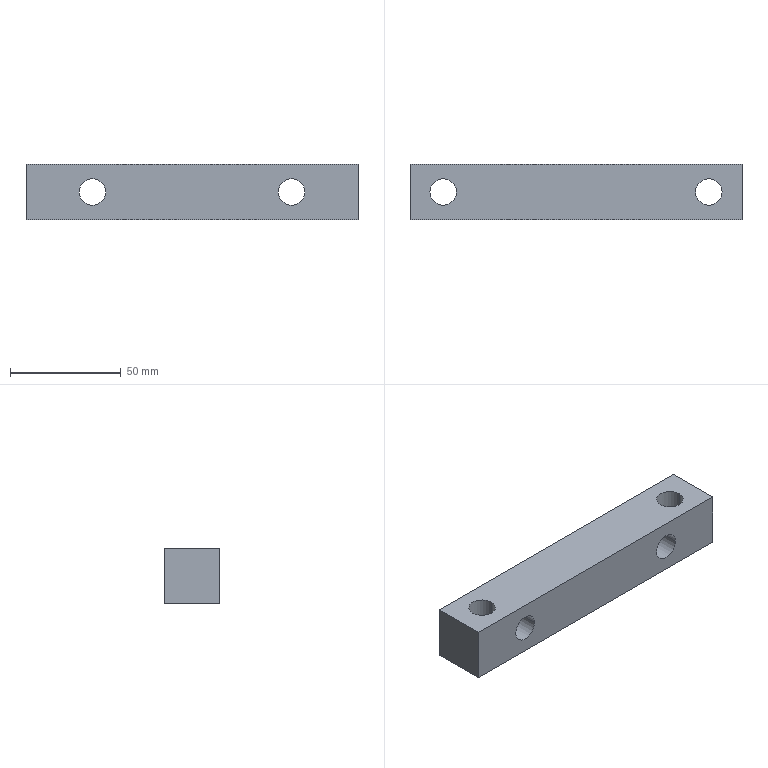Part | STEP file | J013-EBZ05-14-06-Part-1 | 1 solid | 14 faces | box 150 x 25 x 25 mm | volume 82440 mm3 | cylinder 8 | plane 6 | commonest cylinder face diameters 12 x8
STEP:
#1=CARTESIAN_POINT('',(114.,25.,12.5));
#2=VERTEX_POINT('',#1);
#3=CARTESIAN_POINT('',(126.,25.,12.5));
#4=VERTEX_POINT('',#3);
#5=CARTESIAN_POINT('',(120.,25.,12.5));
#6=DIRECTION('',(0.,-1.,0.));
#7=DIRECTION('',(1.,0.,0.));
#8=AXIS2_PLACEMENT_3D('',#5,#6,#7);
#9=CIRCLE('',#8,6.);
#10=EDGE_CURVE('',#2,#4,#9,.T.);
#11=ORIENTED_EDGE('',*,*,#10,.F.);
#12=CARTESIAN_POINT('',(114.,0.,12.5));
#13=VERTEX_POINT('',#12);
#14=CARTESIAN_POINT('',(114.,25.,12.5));
#15=DIRECTION('',(0.,-1.,0.));
#16=VECTOR('',#15,1000.);
#17=LINE('',#14,#16);
#18=EDGE_CURVE('',#2,#13,#17,.T.);
#19=ORIENTED_EDGE('',*,*,#18,.T.);
#20=CARTESIAN_POINT('',(126.,0.,12.5));
#21=VERTEX_POINT('',#20);
#22=CARTESIAN_POINT('',(120.,0.,12.5));
#23=DIRECTION('',(0.,1.,0.));
#24=DIRECTION('',(-1.,0.,0.));
#25=AXIS2_PLACEMENT_3D('',#22,#23,#24);
#26=CIRCLE('',#25,6.);
#27=EDGE_CURVE('',#21,#13,#26,.T.);
#28=ORIENTED_EDGE('',*,*,#27,.F.);
#29=CARTESIAN_POINT('',(126.,25.,12.5));
#30=DIRECTION('',(0.,-1.,0.));
#31=VECTOR('',#30,1000.);
#32=LINE('',#29,#31);
#33=EDGE_CURVE('',#4,#21,#32,.T.);
#34=ORIENTED_EDGE('',*,*,#33,.F.);
#35=EDGE_LOOP('',(#11,#19,#28,#34));
#36=FACE_OUTER_BOUND('',#35,.T.);
#37=CARTESIAN_POINT('',(120.,25.,12.5));
#38=DIRECTION('',(0.,-1.,0.));
#39=DIRECTION('',(1.,0.,0.));
#40=AXIS2_PLACEMENT_3D('',#37,#38,#39);
#41=CYLINDRICAL_SURFACE('',#40,6.);
#42=ADVANCED_FACE('',(#36),#41,.F.);
#43=CARTESIAN_POINT('',(129.,12.5,25.));
#44=VERTEX_POINT('',#43);
#45=CARTESIAN_POINT('',(141.,12.5,25.));
#46=VERTEX_POINT('',#45);
#47=CARTESIAN_POINT('',(135.,12.5,25.));
#48=DIRECTION('',(0.,0.,-1.));
#49=DIRECTION('',(1.,0.,0.));
#50=AXIS2_PLACEMENT_3D('',#47,#48,#49);
#51=CIRCLE('',#50,6.);
#52=EDGE_CURVE('',#44,#46,#51,.T.);
#53=ORIENTED_EDGE('',*,*,#52,.F.);
#54=CARTESIAN_POINT('',(129.,12.5,0.));
#55=VERTEX_POINT('',#54);
#56=CARTESIAN_POINT('',(129.,12.5,25.));
#57=DIRECTION('',(0.,0.,-1.));
#58=VECTOR('',#57,1000.);
#59=LINE('',#56,#58);
#60=EDGE_CURVE('',#44,#55,#59,.T.);
#61=ORIENTED_EDGE('',*,*,#60,.T.);
#62=CARTESIAN_POINT('',(141.,12.5,0.));
#63=VERTEX_POINT('',#62);
#64=CARTESIAN_POINT('',(135.,12.5,0.));
#65=DIRECTION('',(0.,0.,1.));
#66=DIRECTION('',(-1.,0.,0.));
#67=AXIS2_PLACEMENT_3D('',#64,#65,#66);
#68=CIRCLE('',#67,6.);
#69=EDGE_CURVE('',#63,#55,#68,.T.);
#70=ORIENTED_EDGE('',*,*,#69,.F.);
#71=CARTESIAN_POINT('',(141.,12.5,25.));
#72=DIRECTION('',(0.,0.,-1.));
#73=VECTOR('',#72,1000.);
#74=LINE('',#71,#73);
#75=EDGE_CURVE('',#46,#63,#74,.T.);
#76=ORIENTED_EDGE('',*,*,#75,.F.);
#77=EDGE_LOOP('',(#53,#61,#70,#76));
#78=FACE_OUTER_BOUND('',#77,.T.);
#79=CARTESIAN_POINT('',(135.,12.5,25.));
#80=DIRECTION('',(0.,0.,-1.));
#81=DIRECTION('',(1.,0.,0.));
#82=AXIS2_PLACEMENT_3D('',#79,#80,#81);
#83=CYLINDRICAL_SURFACE('',#82,6.);
#84=ADVANCED_FACE('',(#78),#83,.F.);
#85=CARTESIAN_POINT('',(9.,12.5,25.));
#86=VERTEX_POINT('',#85);
#87=CARTESIAN_POINT('',(21.,12.5,25.));
#88=VERTEX_POINT('',#87);
#89=CARTESIAN_POINT('',(15.,12.5,25.));
#90=DIRECTION('',(0.,0.,-1.));
#91=DIRECTION('',(1.,0.,0.));
#92=AXIS2_PLACEMENT_3D('',#89,#90,#91);
#93=CIRCLE('',#92,6.);
#94=EDGE_CURVE('',#86,#88,#93,.T.);
#95=ORIENTED_EDGE('',*,*,#94,.F.);
#96=CARTESIAN_POINT('',(9.,12.5,0.));
#97=VERTEX_POINT('',#96);
#98=CARTESIAN_POINT('',(9.,12.5,25.));
#99=DIRECTION('',(0.,0.,-1.));
#100=VECTOR('',#99,1000.);
#101=LINE('',#98,#100);
#102=EDGE_CURVE('',#86,#97,#101,.T.);
#103=ORIENTED_EDGE('',*,*,#102,.T.);
#104=CARTESIAN_POINT('',(21.,12.5,0.));
#105=VERTEX_POINT('',#104);
#106=CARTESIAN_POINT('',(15.,12.5,0.));
#107=DIRECTION('',(0.,0.,1.));
#108=DIRECTION('',(-1.,0.,0.));
#109=AXIS2_PLACEMENT_3D('',#106,#107,#108);
#110=CIRCLE('',#109,6.);
#111=EDGE_CURVE('',#105,#97,#110,.T.);
#112=ORIENTED_EDGE('',*,*,#111,.F.);
#113=CARTESIAN_POINT('',(21.,12.5,25.));
#114=DIRECTION('',(0.,0.,-1.));
#115=VECTOR('',#114,1000.);
#116=LINE('',#113,#115);
#117=EDGE_CURVE('',#88,#105,#116,.T.);
#118=ORIENTED_EDGE('',*,*,#117,.F.);
#119=EDGE_LOOP('',(#95,#103,#112,#118));
#120=FACE_OUTER_BOUND('',#119,.T.);
#121=CARTESIAN_POINT('',(15.,12.5,25.));
#122=DIRECTION('',(0.,0.,-1.));
#123=DIRECTION('',(1.,0.,0.));
#124=AXIS2_PLACEMENT_3D('',#121,#122,#123);
#125=CYLINDRICAL_SURFACE('',#124,6.);
#126=ADVANCED_FACE('',(#120),#125,.F.);
#127=CARTESIAN_POINT('',(24.,25.,12.5));
#128=VERTEX_POINT('',#127);
#129=CARTESIAN_POINT('',(36.,25.,12.5));
#130=VERTEX_POINT('',#129);
#131=CARTESIAN_POINT('',(30.,25.,12.5));
#132=DIRECTION('',(0.,-1.,0.));
#133=DIRECTION('',(1.,0.,0.));
#134=AXIS2_PLACEMENT_3D('',#131,#132,#133);
#135=CIRCLE('',#134,6.);
#136=EDGE_CURVE('',#128,#130,#135,.T.);
#137=ORIENTED_EDGE('',*,*,#136,.F.);
#138=CARTESIAN_POINT('',(24.,0.,12.5));
#139=VERTEX_POINT('',#138);
#140=CARTESIAN_POINT('',(24.,25.,12.5));
#141=DIRECTION('',(0.,-1.,0.));
#142=VECTOR('',#141,1000.);
#143=LINE('',#140,#142);
#144=EDGE_CURVE('',#128,#139,#143,.T.);
#145=ORIENTED_EDGE('',*,*,#144,.T.);
#146=CARTESIAN_POINT('',(36.,0.,12.5));
#147=VERTEX_POINT('',#146);
#148=CARTESIAN_POINT('',(30.,0.,12.5));
#149=DIRECTION('',(0.,1.,0.));
#150=DIRECTION('',(-1.,0.,0.));
#151=AXIS2_PLACEMENT_3D('',#148,#149,#150);
#152=CIRCLE('',#151,6.);
#153=EDGE_CURVE('',#147,#139,#152,.T.);
#154=ORIENTED_EDGE('',*,*,#153,.F.);
#155=CARTESIAN_POINT('',(36.,25.,12.5));
#156=DIRECTION('',(0.,-1.,0.));
#157=VECTOR('',#156,1000.);
#158=LINE('',#155,#157);
#159=EDGE_CURVE('',#130,#147,#158,.T.);
#160=ORIENTED_EDGE('',*,*,#159,.F.);
#161=EDGE_LOOP('',(#137,#145,#154,#160));
#162=FACE_OUTER_BOUND('',#161,.T.);
#163=CARTESIAN_POINT('',(30.,25.,12.5));
#164=DIRECTION('',(0.,-1.,0.));
#165=DIRECTION('',(1.,0.,0.));
#166=AXIS2_PLACEMENT_3D('',#163,#164,#165);
#167=CYLINDRICAL_SURFACE('',#166,6.);
#168=ADVANCED_FACE('',(#162),#167,.F.);
#169=CARTESIAN_POINT('',(135.,12.5,25.));
#170=DIRECTION('',(0.,0.,-1.));
#171=DIRECTION('',(1.,0.,0.));
#172=AXIS2_PLACEMENT_3D('',#169,#170,#171);
#173=CIRCLE('',#172,6.);
#174=EDGE_CURVE('',#46,#44,#173,.T.);
#175=ORIENTED_EDGE('',*,*,#174,.T.);
#176=ORIENTED_EDGE('',*,*,#52,.T.);
#177=EDGE_LOOP('',(#175,#176));
#178=FACE_BOUND('',#177,.T.);
#179=CARTESIAN_POINT('',(15.,12.5,25.));
#180=DIRECTION('',(0.,0.,-1.));
#181=DIRECTION('',(1.,0.,0.));
#182=AXIS2_PLACEMENT_3D('',#179,#180,#181);
#183=CIRCLE('',#182,6.);
#184=EDGE_CURVE('',#88,#86,#183,.T.);
#185=ORIENTED_EDGE('',*,*,#184,.T.);
#186=ORIENTED_EDGE('',*,*,#94,.T.);
#187=EDGE_LOOP('',(#185,#186));
#188=FACE_BOUND('',#187,.T.);
#189=CARTESIAN_POINT('',(0.,25.,25.));
#190=VERTEX_POINT('',#189);
#191=CARTESIAN_POINT('',(150.,25.,25.));
#192=VERTEX_POINT('',#191);
#193=CARTESIAN_POINT('',(75.,25.,25.));
#194=DIRECTION('',(1.,0.,0.));
#195=VECTOR('',#194,1000.);
#196=LINE('',#193,#195);
#197=EDGE_CURVE('',#190,#192,#196,.T.);
#198=ORIENTED_EDGE('',*,*,#197,.F.);
#199=CARTESIAN_POINT('',(0.,0.,25.));
#200=VERTEX_POINT('',#199);
#201=CARTESIAN_POINT('',(0.,12.5,25.));
#202=DIRECTION('',(0.,1.,0.));
#203=VECTOR('',#202,1000.);
#204=LINE('',#201,#203);
#205=EDGE_CURVE('',#200,#190,#204,.T.);
#206=ORIENTED_EDGE('',*,*,#205,.F.);
#207=CARTESIAN_POINT('',(150.,0.,25.));
#208=VERTEX_POINT('',#207);
#209=CARTESIAN_POINT('',(75.,0.,25.));
#210=DIRECTION('',(-1.,0.,0.));
#211=VECTOR('',#210,1000.);
#212=LINE('',#209,#211);
#213=EDGE_CURVE('',#208,#200,#212,.T.);
#214=ORIENTED_EDGE('',*,*,#213,.F.);
#215=CARTESIAN_POINT('',(150.,12.5,25.));
#216=DIRECTION('',(0.,-1.,0.));
#217=VECTOR('',#216,1000.);
#218=LINE('',#215,#217);
#219=EDGE_CURVE('',#192,#208,#218,.T.);
#220=ORIENTED_EDGE('',*,*,#219,.F.);
#221=EDGE_LOOP('',(#198,#206,#214,#220));
#222=FACE_OUTER_BOUND('',#221,.T.);
#223=CARTESIAN_POINT('',(75.,12.5,25.));
#224=DIRECTION('',(0.,0.,1.));
#225=DIRECTION('',(-1.,0.,0.));
#226=AXIS2_PLACEMENT_3D('',#223,#224,#225);
#227=PLANE('',#226);
#228=ADVANCED_FACE('',(#178,#188,#222),#227,.T.);
#229=CARTESIAN_POINT('',(120.,25.,12.5));
#230=DIRECTION('',(0.,-1.,0.));
#231=DIRECTION('',(1.,0.,0.));
#232=AXIS2_PLACEMENT_3D('',#229,#230,#231);
#233=CIRCLE('',#232,6.);
#234=EDGE_CURVE('',#4,#2,#233,.T.);
#235=ORIENTED_EDGE('',*,*,#234,.T.);
#236=ORIENTED_EDGE('',*,*,#10,.T.);
#237=EDGE_LOOP('',(#235,#236));
#238=FACE_BOUND('',#237,.T.);
#239=CARTESIAN_POINT('',(30.,25.,12.5));
#240=DIRECTION('',(0.,-1.,0.));
#241=DIRECTION('',(1.,0.,0.));
#242=AXIS2_PLACEMENT_3D('',#239,#240,#241);
#243=CIRCLE('',#242,6.);
#244=EDGE_CURVE('',#130,#128,#243,.T.);
#245=ORIENTED_EDGE('',*,*,#244,.T.);
#246=ORIENTED_EDGE('',*,*,#136,.T.);
#247=EDGE_LOOP('',(#245,#246));
#248=FACE_BOUND('',#247,.T.);
#249=CARTESIAN_POINT('',(0.,25.,0.));
#250=VERTEX_POINT('',#249);
#251=CARTESIAN_POINT('',(0.,25.,0.));
#252=DIRECTION('',(0.,0.,1.));
#253=VECTOR('',#252,1000.);
#254=LINE('',#251,#253);
#255=EDGE_CURVE('',#250,#190,#254,.T.);
#256=ORIENTED_EDGE('',*,*,#255,.T.);
#257=ORIENTED_EDGE('',*,*,#197,.T.);
#258=CARTESIAN_POINT('',(150.,25.,0.));
#259=VERTEX_POINT('',#258);
#260=CARTESIAN_POINT('',(150.,25.,0.));
#261=DIRECTION('',(0.,0.,1.));
#262=VECTOR('',#261,1000.);
#263=LINE('',#260,#262);
#264=EDGE_CURVE('',#259,#192,#263,.T.);
#265=ORIENTED_EDGE('',*,*,#264,.F.);
#266=CARTESIAN_POINT('',(75.,25.,0.));
#267=DIRECTION('',(-1.,0.,0.));
#268=VECTOR('',#267,1000.);
#269=LINE('',#266,#268);
#270=EDGE_CURVE('',#259,#250,#269,.T.);
#271=ORIENTED_EDGE('',*,*,#270,.T.);
#272=EDGE_LOOP('',(#256,#257,#265,#271));
#273=FACE_OUTER_BOUND('',#272,.T.);
#274=CARTESIAN_POINT('',(75.,25.,0.));
#275=DIRECTION('',(0.,1.,0.));
#276=DIRECTION('',(0.,0.,-1.));
#277=AXIS2_PLACEMENT_3D('',#274,#275,#276);
#278=PLANE('',#277);
#279=ADVANCED_FACE('',(#238,#248,#273),#278,.T.);
#280=ORIENTED_EDGE('',*,*,#264,.T.);
#281=ORIENTED_EDGE('',*,*,#219,.T.);
#282=CARTESIAN_POINT('',(150.,0.,0.));
#283=VERTEX_POINT('',#282);
#284=CARTESIAN_POINT('',(150.,0.,0.));
#285=DIRECTION('',(0.,0.,1.));
#286=VECTOR('',#285,1000.);
#287=LINE('',#284,#286);
#288=EDGE_CURVE('',#283,#208,#287,.T.);
#289=ORIENTED_EDGE('',*,*,#288,.F.);
#290=CARTESIAN_POINT('',(150.,12.5,0.));
#291=DIRECTION('',(0.,1.,0.));
#292=VECTOR('',#291,1000.);
#293=LINE('',#290,#292);
#294=EDGE_CURVE('',#283,#259,#293,.T.);
#295=ORIENTED_EDGE('',*,*,#294,.T.);
#296=EDGE_LOOP('',(#280,#281,#289,#295));
#297=FACE_OUTER_BOUND('',#296,.T.);
#298=CARTESIAN_POINT('',(150.,12.5,0.));
#299=DIRECTION('',(1.,0.,0.));
#300=DIRECTION('',(0.,0.,1.));
#301=AXIS2_PLACEMENT_3D('',#298,#299,#300);
#302=PLANE('',#301);
#303=ADVANCED_FACE('',(#297),#302,.T.);
#304=ORIENTED_EDGE('',*,*,#27,.T.);
#305=CARTESIAN_POINT('',(120.,0.,12.5));
#306=DIRECTION('',(0.,1.,0.));
#307=DIRECTION('',(-1.,0.,0.));
#308=AXIS2_PLACEMENT_3D('',#305,#306,#307);
#309=CIRCLE('',#308,6.);
#310=EDGE_CURVE('',#13,#21,#309,.T.);
#311=ORIENTED_EDGE('',*,*,#310,.T.);
#312=EDGE_LOOP('',(#304,#311));
#313=FACE_BOUND('',#312,.T.);
#314=ORIENTED_EDGE('',*,*,#153,.T.);
#315=CARTESIAN_POINT('',(30.,0.,12.5));
#316=DIRECTION('',(0.,1.,0.));
#317=DIRECTION('',(-1.,0.,0.));
#318=AXIS2_PLACEMENT_3D('',#315,#316,#317);
#319=CIRCLE('',#318,6.);
#320=EDGE_CURVE('',#139,#147,#319,.T.);
#321=ORIENTED_EDGE('',*,*,#320,.T.);
#322=EDGE_LOOP('',(#314,#321));
#323=FACE_BOUND('',#322,.T.);
#324=ORIENTED_EDGE('',*,*,#288,.T.);
#325=ORIENTED_EDGE('',*,*,#213,.T.);
#326=CARTESIAN_POINT('',(0.,0.,0.));
#327=VERTEX_POINT('',#326);
#328=CARTESIAN_POINT('',(0.,0.,0.));
#329=DIRECTION('',(0.,0.,1.));
#330=VECTOR('',#329,1000.);
#331=LINE('',#328,#330);
#332=EDGE_CURVE('',#327,#200,#331,.T.);
#333=ORIENTED_EDGE('',*,*,#332,.F.);
#334=CARTESIAN_POINT('',(75.,0.,0.));
#335=DIRECTION('',(1.,0.,0.));
#336=VECTOR('',#335,1000.);
#337=LINE('',#334,#336);
#338=EDGE_CURVE('',#327,#283,#337,.T.);
#339=ORIENTED_EDGE('',*,*,#338,.T.);
#340=EDGE_LOOP('',(#324,#325,#333,#339));
#341=FACE_OUTER_BOUND('',#340,.T.);
#342=CARTESIAN_POINT('',(75.,0.,0.));
#343=DIRECTION('',(0.,-1.,0.));
#344=DIRECTION('',(0.,0.,1.));
#345=AXIS2_PLACEMENT_3D('',#342,#343,#344);
#346=PLANE('',#345);
#347=ADVANCED_FACE('',(#313,#323,#341),#346,.T.);
#348=ORIENTED_EDGE('',*,*,#69,.T.);
#349=CARTESIAN_POINT('',(135.,12.5,0.));
#350=DIRECTION('',(0.,0.,1.));
#351=DIRECTION('',(-1.,0.,0.));
#352=AXIS2_PLACEMENT_3D('',#349,#350,#351);
#353=CIRCLE('',#352,6.);
#354=EDGE_CURVE('',#55,#63,#353,.T.);
#355=ORIENTED_EDGE('',*,*,#354,.T.);
#356=EDGE_LOOP('',(#348,#355));
#357=FACE_BOUND('',#356,.T.);
#358=ORIENTED_EDGE('',*,*,#111,.T.);
#359=CARTESIAN_POINT('',(15.,12.5,0.));
#360=DIRECTION('',(0.,0.,1.));
#361=DIRECTION('',(-1.,0.,0.));
#362=AXIS2_PLACEMENT_3D('',#359,#360,#361);
#363=CIRCLE('',#362,6.);
#364=EDGE_CURVE('',#97,#105,#363,.T.);
#365=ORIENTED_EDGE('',*,*,#364,.T.);
#366=EDGE_LOOP('',(#358,#365));
#367=FACE_BOUND('',#366,.T.);
#368=CARTESIAN_POINT('',(0.,12.5,0.));
#369=DIRECTION('',(0.,-1.,0.));
#370=VECTOR('',#369,1000.);
#371=LINE('',#368,#370);
#372=EDGE_CURVE('',#250,#327,#371,.T.);
#373=ORIENTED_EDGE('',*,*,#372,.F.);
#374=ORIENTED_EDGE('',*,*,#270,.F.);
#375=ORIENTED_EDGE('',*,*,#294,.F.);
#376=ORIENTED_EDGE('',*,*,#338,.F.);
#377=EDGE_LOOP('',(#373,#374,#375,#376));
#378=FACE_OUTER_BOUND('',#377,.T.);
#379=CARTESIAN_POINT('',(75.,12.5,0.));
#380=DIRECTION('',(0.,0.,-1.));
#381=DIRECTION('',(1.,0.,0.));
#382=AXIS2_PLACEMENT_3D('',#379,#380,#381);
#383=PLANE('',#382);
#384=ADVANCED_FACE('',(#357,#367,#378),#383,.T.);
#385=ORIENTED_EDGE('',*,*,#372,.T.);
#386=ORIENTED_EDGE('',*,*,#332,.T.);
#387=ORIENTED_EDGE('',*,*,#205,.T.);
#388=ORIENTED_EDGE('',*,*,#255,.F.);
#389=EDGE_LOOP('',(#385,#386,#387,#388));
#390=FACE_OUTER_BOUND('',#389,.T.);
#391=CARTESIAN_POINT('',(0.,12.5,0.));
#392=DIRECTION('',(-1.,0.,0.));
#393=DIRECTION('',(0.,0.,-1.));
#394=AXIS2_PLACEMENT_3D('',#391,#392,#393);
#395=PLANE('',#394);
#396=ADVANCED_FACE('',(#390),#395,.T.);
#397=ORIENTED_EDGE('',*,*,#144,.F.);
#398=ORIENTED_EDGE('',*,*,#244,.F.);
#399=ORIENTED_EDGE('',*,*,#159,.T.);
#400=ORIENTED_EDGE('',*,*,#320,.F.);
#401=EDGE_LOOP('',(#397,#398,#399,#400));
#402=FACE_OUTER_BOUND('',#401,.T.);
#403=CARTESIAN_POINT('',(30.,25.,12.5));
#404=DIRECTION('',(0.,-1.,0.));
#405=DIRECTION('',(1.,0.,0.));
#406=AXIS2_PLACEMENT_3D('',#403,#404,#405);
#407=CYLINDRICAL_SURFACE('',#406,6.);
#408=ADVANCED_FACE('',(#402),#407,.F.);
#409=ORIENTED_EDGE('',*,*,#102,.F.);
#410=ORIENTED_EDGE('',*,*,#184,.F.);
#411=ORIENTED_EDGE('',*,*,#117,.T.);
#412=ORIENTED_EDGE('',*,*,#364,.F.);
#413=EDGE_LOOP('',(#409,#410,#411,#412));
#414=FACE_OUTER_BOUND('',#413,.T.);
#415=CARTESIAN_POINT('',(15.,12.5,25.));
#416=DIRECTION('',(0.,0.,-1.));
#417=DIRECTION('',(1.,0.,0.));
#418=AXIS2_PLACEMENT_3D('',#415,#416,#417);
#419=CYLINDRICAL_SURFACE('',#418,6.);
#420=ADVANCED_FACE('',(#414),#419,.F.);
#421=ORIENTED_EDGE('',*,*,#60,.F.);
#422=ORIENTED_EDGE('',*,*,#174,.F.);
#423=ORIENTED_EDGE('',*,*,#75,.T.);
#424=ORIENTED_EDGE('',*,*,#354,.F.);
#425=EDGE_LOOP('',(#421,#422,#423,#424));
#426=FACE_OUTER_BOUND('',#425,.T.);
#427=CARTESIAN_POINT('',(135.,12.5,25.));
#428=DIRECTION('',(0.,0.,-1.));
#429=DIRECTION('',(1.,0.,0.));
#430=AXIS2_PLACEMENT_3D('',#427,#428,#429);
#431=CYLINDRICAL_SURFACE('',#430,6.);
#432=ADVANCED_FACE('',(#426),#431,.F.);
#433=ORIENTED_EDGE('',*,*,#18,.F.);
#434=ORIENTED_EDGE('',*,*,#234,.F.);
#435=ORIENTED_EDGE('',*,*,#33,.T.);
#436=ORIENTED_EDGE('',*,*,#310,.F.);
#437=EDGE_LOOP('',(#433,#434,#435,#436));
#438=FACE_OUTER_BOUND('',#437,.T.);
#439=CARTESIAN_POINT('',(120.,25.,12.5));
#440=DIRECTION('',(0.,-1.,0.));
#441=DIRECTION('',(1.,0.,0.));
#442=AXIS2_PLACEMENT_3D('',#439,#440,#441);
#443=CYLINDRICAL_SURFACE('',#442,6.);
#444=ADVANCED_FACE('',(#438),#443,.F.);
#445=CLOSED_SHELL('',(#42,#84,#126,#168,#228,#279,#303,#347,#384,#396,#408,#420,#432,#444));
#446=MANIFOLD_SOLID_BREP('',#445);
#447=CARTESIAN_POINT('',(0.,0.,0.));
#448=DIRECTION('',(0.,0.,1.));
#449=DIRECTION('',(1.,0.,0.));
#450=AXIS2_PLACEMENT_3D('',#447,#448,#449);
#451=(LENGTH_UNIT()NAMED_UNIT(*)SI_UNIT(.MILLI.,.METRE.));
#452=UNCERTAINTY_MEASURE_WITH_UNIT(LENGTH_MEASURE(0.00001),#451,'','');
#453=(NAMED_UNIT(*)PLANE_ANGLE_UNIT()SI_UNIT($,.RADIAN.));
#454=(NAMED_UNIT(*)SI_UNIT($,.STERADIAN.)SOLID_ANGLE_UNIT());
#455=(GEOMETRIC_REPRESENTATION_CONTEXT(3)GLOBAL_UNCERTAINTY_ASSIGNED_CONTEXT((#452))GLOBAL_UNIT_ASSIGNED_CONTEXT((#451,#453,#454))REPRESENTATION_CONTEXT('',''));
#456=ADVANCED_BREP_SHAPE_REPRESENTATION('',(#446,#450),#455);